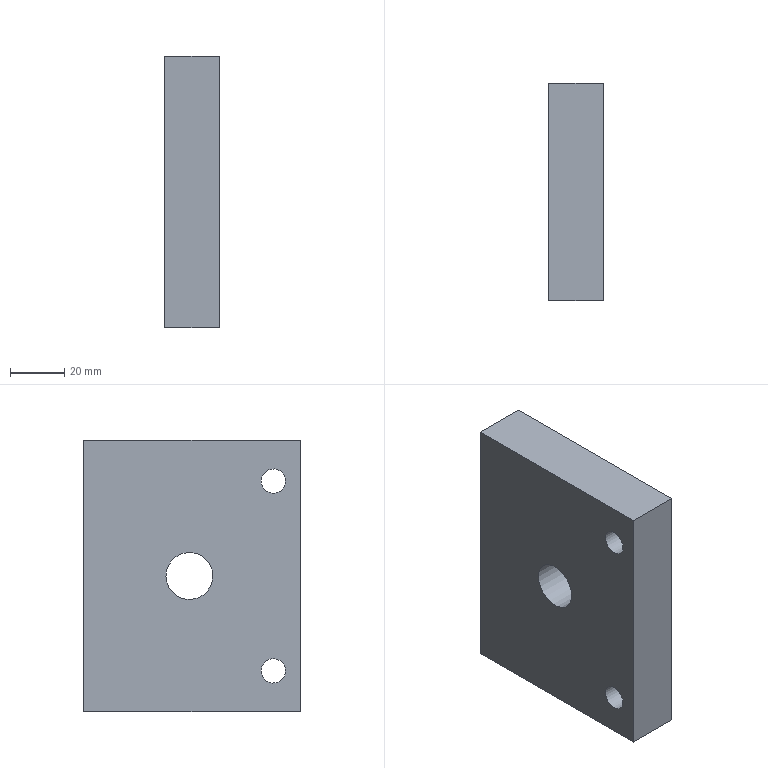Part | STEP file | SN10_001_004_PLACA | 1 solid | 9 faces | box 20 x 80 x 100 mm | volume 152757 mm3 | plane 6 | cylinder 3 | commonest cylinder face diameters 9 x2 17.294 x1
STEP:
#1=CARTESIAN_POINT('',(0.,0.,0.));
#2=DIRECTION('',(0.,0.,1.));
#3=DIRECTION('',(1.,0.,0.));
#4=AXIS2_PLACEMENT_3D('',#1,#2,#3);
#5=CARTESIAN_POINT('',(320.,193.949,32.843));
#6=VERTEX_POINT('',#5);
#7=CARTESIAN_POINT('',(320.,190.,35.));
#8=DIRECTION('',(-1.,0.,0.));
#9=DIRECTION('',(0.,1.,0.));
#10=AXIS2_PLACEMENT_3D('',#7,#8,#9);
#11=CIRCLE('',#10,4.5);
#12=CARTESIAN_POINT('',(319.9,190.,35.));
#13=DIRECTION('',(-1.,0.,0.));
#14=DIRECTION('',(0.,0.8776,-0.4794));
#15=AXIS2_PLACEMENT_3D('',#12,#13,#14);
#16=CYLINDRICAL_SURFACE('',#15,4.5);
#17=CARTESIAN_POINT('',(-0.5,-0.1));
#18=DIRECTION('',(1.,0.));
#19=VECTOR('',#18,1.);
#20=LINE('',#17,#19);
#21=(GEOMETRIC_REPRESENTATION_CONTEXT(2)PARAMETRIC_REPRESENTATION_CONTEXT()REPRESENTATION_CONTEXT('',''));
#22=DEFINITIONAL_REPRESENTATION('',(#20),#21);
#23=PCURVE('',#16,#22);
#24=CARTESIAN_POINT('',(320.,180.,0.));
#25=DIRECTION('',(1.,0.,0.));
#26=DIRECTION('',(0.,0.,-1.));
#27=AXIS2_PLACEMENT_3D('',#24,#25,#26);
#28=PLANE('',#27);
#29=CARTESIAN_POINT('',(-35.,14.5));
#30=CARTESIAN_POINT('',(-27.206,14.5));
#31=CARTESIAN_POINT('',(-31.103,7.75));
#32=CARTESIAN_POINT('',(-35.,1.));
#33=CARTESIAN_POINT('',(-38.897,7.75));
#34=CARTESIAN_POINT('',(-42.794,14.5));
#35=CARTESIAN_POINT('',(-35.,14.5));
#36=(BOUNDED_CURVE()B_SPLINE_CURVE(2,(#29,#30,#31,#32,#33,#34,#35),.UNSPECIFIED.,.T.,.F.)B_SPLINE_CURVE_WITH_KNOTS((1,2,2,2,2,1),(-2.094,0.,2.094,4.189,6.283,8.378),.UNSPECIFIED.)CURVE()GEOMETRIC_REPRESENTATION_ITEM()RATIONAL_B_SPLINE_CURVE((1.,0.5,1.,0.5,1.,0.5,1.))REPRESENTATION_ITEM(''));
#37=(GEOMETRIC_REPRESENTATION_CONTEXT(2)PARAMETRIC_REPRESENTATION_CONTEXT()REPRESENTATION_CONTEXT('',''));
#38=DEFINITIONAL_REPRESENTATION('',(#36),#37);
#39=PCURVE('',#28,#38);
#40=SURFACE_CURVE('',#11,(#23,#39),.PCURVE_S1.);
#41=EDGE_CURVE('',#6,#6,#40,.T.);
#42=ORIENTED_EDGE('',*,*,#41,.T.);
#43=CARTESIAN_POINT('',(300.,193.949,32.843));
#44=VERTEX_POINT('',#43);
#45=CARTESIAN_POINT('',(320.,193.949,32.843));
#46=CARTESIAN_POINT('',(300.,193.949,32.843));
#47=B_SPLINE_CURVE_WITH_KNOTS('',1,(#45,#46),.UNSPECIFIED.,.F.,.F.,(2,2),(-0.1,19.9),.PIECEWISE_BEZIER_KNOTS.);
#48=CARTESIAN_POINT('',(6.283,0.));
#49=DIRECTION('',(0.,1.));
#50=VECTOR('',#49,1.);
#51=LINE('',#48,#50);
#52=(GEOMETRIC_REPRESENTATION_CONTEXT(2)PARAMETRIC_REPRESENTATION_CONTEXT()REPRESENTATION_CONTEXT('',''));
#53=DEFINITIONAL_REPRESENTATION('',(#51),#52);
#54=PCURVE('',#16,#53);
#55=CARTESIAN_POINT('',(0.,0.));
#56=DIRECTION('',(0.,1.));
#57=VECTOR('',#56,1.);
#58=LINE('',#55,#57);
#59=(GEOMETRIC_REPRESENTATION_CONTEXT(2)PARAMETRIC_REPRESENTATION_CONTEXT()REPRESENTATION_CONTEXT('',''));
#60=DEFINITIONAL_REPRESENTATION('',(#58),#59);
#61=PCURVE('',#16,#60);
#62=SEAM_CURVE('',#47,(#54,#61),.PCURVE_S1.);
#63=EDGE_CURVE('',#6,#44,#62,.T.);
#64=ORIENTED_EDGE('',*,*,#63,.T.);
#65=CARTESIAN_POINT('',(300.,190.,35.));
#66=DIRECTION('',(-1.,0.,0.));
#67=DIRECTION('',(0.,1.,0.));
#68=AXIS2_PLACEMENT_3D('',#65,#66,#67);
#69=CIRCLE('',#68,4.5);
#70=CARTESIAN_POINT('',(-0.5,19.9));
#71=DIRECTION('',(1.,0.));
#72=VECTOR('',#71,1.);
#73=LINE('',#70,#72);
#74=(GEOMETRIC_REPRESENTATION_CONTEXT(2)PARAMETRIC_REPRESENTATION_CONTEXT()REPRESENTATION_CONTEXT('',''));
#75=DEFINITIONAL_REPRESENTATION('',(#73),#74);
#76=PCURVE('',#16,#75);
#77=CARTESIAN_POINT('',(300.,260.,0.));
#78=DIRECTION('',(-1.,0.,0.));
#79=DIRECTION('',(0.,0.,1.));
#80=AXIS2_PLACEMENT_3D('',#77,#78,#79);
#81=PLANE('',#80);
#82=CARTESIAN_POINT('',(35.,-70.));
#83=DIRECTION('',(0.,1.));
#84=AXIS2_PLACEMENT_2D('',#82,#83);
#85=CIRCLE('',#84,4.5);
#86=(GEOMETRIC_REPRESENTATION_CONTEXT(2)PARAMETRIC_REPRESENTATION_CONTEXT()REPRESENTATION_CONTEXT('',''));
#87=DEFINITIONAL_REPRESENTATION('',(#85),#86);
#88=PCURVE('',#81,#87);
#89=SURFACE_CURVE('',#69,(#76,#88),.PCURVE_S1.);
#90=EDGE_CURVE('',#44,#44,#89,.T.);
#91=ORIENTED_EDGE('',*,*,#90,.F.);
#92=ORIENTED_EDGE('',*,*,#63,.F.);
#93=EDGE_LOOP('',(#42,#64,#91,#92));
#94=FACE_BOUND('',#93,.F.);
#95=ADVANCED_FACE('',(#94),#16,.F.);
#96=CARTESIAN_POINT('',(320.,260.,-50.));
#97=VERTEX_POINT('',#96);
#98=CARTESIAN_POINT('',(300.,260.,-50.));
#99=VERTEX_POINT('',#98);
#100=CARTESIAN_POINT('',(320.,260.,-50.));
#101=DIRECTION('',(-1.,0.,0.));
#102=VECTOR('',#101,1.);
#103=LINE('',#100,#102);
#104=CARTESIAN_POINT('',(0.,0.,-50.));
#105=DIRECTION('',(0.,0.,1.));
#106=DIRECTION('',(1.,0.,0.));
#107=AXIS2_PLACEMENT_3D('',#104,#105,#106);
#108=PLANE('',#107);
#109=CARTESIAN_POINT('',(320.,260.));
#110=DIRECTION('',(-1.,0.));
#111=VECTOR('',#110,1.);
#112=LINE('',#109,#111);
#113=(GEOMETRIC_REPRESENTATION_CONTEXT(2)PARAMETRIC_REPRESENTATION_CONTEXT()REPRESENTATION_CONTEXT('',''));
#114=DEFINITIONAL_REPRESENTATION('',(#112),#113);
#115=PCURVE('',#108,#114);
#116=CARTESIAN_POINT('',(320.,260.,0.));
#117=DIRECTION('',(0.,1.,0.));
#118=DIRECTION('',(0.,0.,1.));
#119=AXIS2_PLACEMENT_3D('',#116,#117,#118);
#120=PLANE('',#119);
#121=CARTESIAN_POINT('',(-50.,0.));
#122=DIRECTION('',(0.,-1.));
#123=VECTOR('',#122,1.);
#124=LINE('',#121,#123);
#125=(GEOMETRIC_REPRESENTATION_CONTEXT(2)PARAMETRIC_REPRESENTATION_CONTEXT()REPRESENTATION_CONTEXT('',''));
#126=DEFINITIONAL_REPRESENTATION('',(#124),#125);
#127=PCURVE('',#120,#126);
#128=SURFACE_CURVE('',#103,(#115,#127),.PCURVE_S1.);
#129=EDGE_CURVE('',#97,#99,#128,.T.);
#130=ORIENTED_EDGE('',*,*,#129,.F.);
#131=CARTESIAN_POINT('',(320.,180.,-50.));
#132=VERTEX_POINT('',#131);
#133=CARTESIAN_POINT('',(320.,180.,-50.));
#134=DIRECTION('',(0.,1.,0.));
#135=VECTOR('',#134,1.);
#136=LINE('',#133,#135);
#137=CARTESIAN_POINT('',(320.,180.));
#138=DIRECTION('',(0.,1.));
#139=VECTOR('',#138,1.);
#140=LINE('',#137,#139);
#141=(GEOMETRIC_REPRESENTATION_CONTEXT(2)PARAMETRIC_REPRESENTATION_CONTEXT()REPRESENTATION_CONTEXT('',''));
#142=DEFINITIONAL_REPRESENTATION('',(#140),#141);
#143=PCURVE('',#108,#142);
#144=CARTESIAN_POINT('',(50.,0.));
#145=DIRECTION('',(0.,1.));
#146=VECTOR('',#145,1.);
#147=LINE('',#144,#146);
#148=(GEOMETRIC_REPRESENTATION_CONTEXT(2)PARAMETRIC_REPRESENTATION_CONTEXT()REPRESENTATION_CONTEXT('',''));
#149=DEFINITIONAL_REPRESENTATION('',(#147),#148);
#150=PCURVE('',#28,#149);
#151=SURFACE_CURVE('',#136,(#143,#150),.PCURVE_S1.);
#152=EDGE_CURVE('',#132,#97,#151,.T.);
#153=ORIENTED_EDGE('',*,*,#152,.F.);
#154=CARTESIAN_POINT('',(300.,180.,-50.));
#155=VERTEX_POINT('',#154);
#156=CARTESIAN_POINT('',(300.,180.,-50.));
#157=DIRECTION('',(1.,0.,0.));
#158=VECTOR('',#157,1.);
#159=LINE('',#156,#158);
#160=CARTESIAN_POINT('',(300.,180.));
#161=DIRECTION('',(1.,0.));
#162=VECTOR('',#161,1.);
#163=LINE('',#160,#162);
#164=(GEOMETRIC_REPRESENTATION_CONTEXT(2)PARAMETRIC_REPRESENTATION_CONTEXT()REPRESENTATION_CONTEXT('',''));
#165=DEFINITIONAL_REPRESENTATION('',(#163),#164);
#166=PCURVE('',#108,#165);
#167=CARTESIAN_POINT('',(300.,180.,0.));
#168=DIRECTION('',(0.,-1.,0.));
#169=DIRECTION('',(0.,0.,-1.));
#170=AXIS2_PLACEMENT_3D('',#167,#168,#169);
#171=PLANE('',#170);
#172=CARTESIAN_POINT('',(50.,0.));
#173=DIRECTION('',(0.,1.));
#174=VECTOR('',#173,1.);
#175=LINE('',#172,#174);
#176=(GEOMETRIC_REPRESENTATION_CONTEXT(2)PARAMETRIC_REPRESENTATION_CONTEXT()REPRESENTATION_CONTEXT('',''));
#177=DEFINITIONAL_REPRESENTATION('',(#175),#176);
#178=PCURVE('',#171,#177);
#179=SURFACE_CURVE('',#159,(#166,#178),.PCURVE_S1.);
#180=EDGE_CURVE('',#155,#132,#179,.T.);
#181=ORIENTED_EDGE('',*,*,#180,.F.);
#182=CARTESIAN_POINT('',(300.,260.,-50.));
#183=DIRECTION('',(0.,-1.,0.));
#184=VECTOR('',#183,1.);
#185=LINE('',#182,#184);
#186=CARTESIAN_POINT('',(300.,260.));
#187=DIRECTION('',(0.,-1.));
#188=VECTOR('',#187,1.);
#189=LINE('',#186,#188);
#190=(GEOMETRIC_REPRESENTATION_CONTEXT(2)PARAMETRIC_REPRESENTATION_CONTEXT()REPRESENTATION_CONTEXT('',''));
#191=DEFINITIONAL_REPRESENTATION('',(#189),#190);
#192=PCURVE('',#108,#191);
#193=CARTESIAN_POINT('',(-50.,0.));
#194=DIRECTION('',(0.,-1.));
#195=VECTOR('',#194,1.);
#196=LINE('',#193,#195);
#197=(GEOMETRIC_REPRESENTATION_CONTEXT(2)PARAMETRIC_REPRESENTATION_CONTEXT()REPRESENTATION_CONTEXT('',''));
#198=DEFINITIONAL_REPRESENTATION('',(#196),#197);
#199=PCURVE('',#81,#198);
#200=SURFACE_CURVE('',#185,(#192,#199),.PCURVE_S1.);
#201=EDGE_CURVE('',#99,#155,#200,.T.);
#202=ORIENTED_EDGE('',*,*,#201,.F.);
#203=EDGE_LOOP('',(#130,#153,#181,#202));
#204=FACE_BOUND('',#203,.T.);
#205=ADVANCED_FACE('',(#204),#108,.F.);
#206=CARTESIAN_POINT('',(320.,260.,50.));
#207=VERTEX_POINT('',#206);
#208=CARTESIAN_POINT('',(320.,260.,-50.));
#209=DIRECTION('',(0.,0.,1.));
#210=VECTOR('',#209,1.);
#211=LINE('',#208,#210);
#212=CARTESIAN_POINT('',(-50.,0.));
#213=DIRECTION('',(1.,0.));
#214=VECTOR('',#213,1.);
#215=LINE('',#212,#214);
#216=(GEOMETRIC_REPRESENTATION_CONTEXT(2)PARAMETRIC_REPRESENTATION_CONTEXT()REPRESENTATION_CONTEXT('',''));
#217=DEFINITIONAL_REPRESENTATION('',(#215),#216);
#218=PCURVE('',#120,#217);
#219=CARTESIAN_POINT('',(50.,80.));
#220=DIRECTION('',(-1.,0.));
#221=VECTOR('',#220,1.);
#222=LINE('',#219,#221);
#223=(GEOMETRIC_REPRESENTATION_CONTEXT(2)PARAMETRIC_REPRESENTATION_CONTEXT()REPRESENTATION_CONTEXT('',''));
#224=DEFINITIONAL_REPRESENTATION('',(#222),#223);
#225=PCURVE('',#28,#224);
#226=SURFACE_CURVE('',#211,(#218,#225),.PCURVE_S1.);
#227=EDGE_CURVE('',#97,#207,#226,.T.);
#228=ORIENTED_EDGE('',*,*,#227,.F.);
#229=ORIENTED_EDGE('',*,*,#129,.T.);
#230=CARTESIAN_POINT('',(300.,260.,50.));
#231=VERTEX_POINT('',#230);
#232=CARTESIAN_POINT('',(300.,260.,-50.));
#233=DIRECTION('',(0.,0.,1.));
#234=VECTOR('',#233,1.);
#235=LINE('',#232,#234);
#236=CARTESIAN_POINT('',(-50.,-20.));
#237=DIRECTION('',(1.,0.));
#238=VECTOR('',#237,1.);
#239=LINE('',#236,#238);
#240=(GEOMETRIC_REPRESENTATION_CONTEXT(2)PARAMETRIC_REPRESENTATION_CONTEXT()REPRESENTATION_CONTEXT('',''));
#241=DEFINITIONAL_REPRESENTATION('',(#239),#240);
#242=PCURVE('',#120,#241);
#243=CARTESIAN_POINT('',(-50.,0.));
#244=DIRECTION('',(1.,0.));
#245=VECTOR('',#244,1.);
#246=LINE('',#243,#245);
#247=(GEOMETRIC_REPRESENTATION_CONTEXT(2)PARAMETRIC_REPRESENTATION_CONTEXT()REPRESENTATION_CONTEXT('',''));
#248=DEFINITIONAL_REPRESENTATION('',(#246),#247);
#249=PCURVE('',#81,#248);
#250=SURFACE_CURVE('',#235,(#242,#249),.PCURVE_S1.);
#251=EDGE_CURVE('',#99,#231,#250,.T.);
#252=ORIENTED_EDGE('',*,*,#251,.T.);
#253=CARTESIAN_POINT('',(320.,260.,50.));
#254=DIRECTION('',(-1.,0.,0.));
#255=VECTOR('',#254,1.);
#256=LINE('',#253,#255);
#257=CARTESIAN_POINT('',(50.,0.));
#258=DIRECTION('',(0.,-1.));
#259=VECTOR('',#258,1.);
#260=LINE('',#257,#259);
#261=(GEOMETRIC_REPRESENTATION_CONTEXT(2)PARAMETRIC_REPRESENTATION_CONTEXT()REPRESENTATION_CONTEXT('',''));
#262=DEFINITIONAL_REPRESENTATION('',(#260),#261);
#263=PCURVE('',#120,#262);
#264=CARTESIAN_POINT('',(0.,0.,50.));
#265=DIRECTION('',(0.,0.,1.));
#266=DIRECTION('',(1.,0.,0.));
#267=AXIS2_PLACEMENT_3D('',#264,#265,#266);
#268=PLANE('',#267);
#269=CARTESIAN_POINT('',(320.,260.));
#270=DIRECTION('',(-1.,0.));
#271=VECTOR('',#270,1.);
#272=LINE('',#269,#271);
#273=(GEOMETRIC_REPRESENTATION_CONTEXT(2)PARAMETRIC_REPRESENTATION_CONTEXT()REPRESENTATION_CONTEXT('',''));
#274=DEFINITIONAL_REPRESENTATION('',(#272),#273);
#275=PCURVE('',#268,#274);
#276=SURFACE_CURVE('',#256,(#263,#275),.PCURVE_S1.);
#277=EDGE_CURVE('',#207,#231,#276,.T.);
#278=ORIENTED_EDGE('',*,*,#277,.F.);
#279=EDGE_LOOP('',(#228,#229,#252,#278));
#280=FACE_BOUND('',#279,.T.);
#281=ADVANCED_FACE('',(#280),#120,.T.);
#282=CARTESIAN_POINT('',(320.,228.538,-4.146));
#283=VERTEX_POINT('',#282);
#284=CARTESIAN_POINT('',(320.,220.95,0.));
#285=DIRECTION('',(-1.,0.,0.));
#286=DIRECTION('',(0.,1.,0.));
#287=AXIS2_PLACEMENT_3D('',#284,#285,#286);
#288=CIRCLE('',#287,8.647);
#289=CARTESIAN_POINT('',(319.9,220.95,0.));
#290=DIRECTION('',(-1.,0.,0.));
#291=DIRECTION('',(0.,0.8776,-0.4794));
#292=AXIS2_PLACEMENT_3D('',#289,#290,#291);
#293=CYLINDRICAL_SURFACE('',#292,8.647);
#294=CARTESIAN_POINT('',(-0.5,-0.1));
#295=DIRECTION('',(1.,0.));
#296=VECTOR('',#295,1.);
#297=LINE('',#294,#296);
#298=(GEOMETRIC_REPRESENTATION_CONTEXT(2)PARAMETRIC_REPRESENTATION_CONTEXT()REPRESENTATION_CONTEXT('',''));
#299=DEFINITIONAL_REPRESENTATION('',(#297),#298);
#300=PCURVE('',#293,#299);
#301=CARTESIAN_POINT('',(0.,49.597));
#302=CARTESIAN_POINT('',(14.977,49.597));
#303=CARTESIAN_POINT('',(7.489,36.627));
#304=CARTESIAN_POINT('',(0.,23.656));
#305=CARTESIAN_POINT('',(-7.489,36.627));
#306=CARTESIAN_POINT('',(-14.977,49.597));
#307=CARTESIAN_POINT('',(0.,49.597));
#308=(BOUNDED_CURVE()B_SPLINE_CURVE(2,(#301,#302,#303,#304,#305,#306,#307),.UNSPECIFIED.,.T.,.F.)B_SPLINE_CURVE_WITH_KNOTS((1,2,2,2,2,1),(-2.094,0.,2.094,4.189,6.283,8.378),.UNSPECIFIED.)CURVE()GEOMETRIC_REPRESENTATION_ITEM()RATIONAL_B_SPLINE_CURVE((1.,0.5,1.,0.5,1.,0.5,1.))REPRESENTATION_ITEM(''));
#309=(GEOMETRIC_REPRESENTATION_CONTEXT(2)PARAMETRIC_REPRESENTATION_CONTEXT()REPRESENTATION_CONTEXT('',''));
#310=DEFINITIONAL_REPRESENTATION('',(#308),#309);
#311=PCURVE('',#28,#310);
#312=SURFACE_CURVE('',#288,(#300,#311),.PCURVE_S1.);
#313=EDGE_CURVE('',#283,#283,#312,.T.);
#314=ORIENTED_EDGE('',*,*,#313,.T.);
#315=CARTESIAN_POINT('',(300.,228.538,-4.146));
#316=VERTEX_POINT('',#315);
#317=CARTESIAN_POINT('',(320.,228.538,-4.146));
#318=CARTESIAN_POINT('',(300.,228.538,-4.146));
#319=B_SPLINE_CURVE_WITH_KNOTS('',1,(#317,#318),.UNSPECIFIED.,.F.,.F.,(2,2),(-0.1,19.9),.PIECEWISE_BEZIER_KNOTS.);
#320=CARTESIAN_POINT('',(6.283,0.));
#321=DIRECTION('',(0.,1.));
#322=VECTOR('',#321,1.);
#323=LINE('',#320,#322);
#324=(GEOMETRIC_REPRESENTATION_CONTEXT(2)PARAMETRIC_REPRESENTATION_CONTEXT()REPRESENTATION_CONTEXT('',''));
#325=DEFINITIONAL_REPRESENTATION('',(#323),#324);
#326=PCURVE('',#293,#325);
#327=CARTESIAN_POINT('',(0.,0.));
#328=DIRECTION('',(0.,1.));
#329=VECTOR('',#328,1.);
#330=LINE('',#327,#329);
#331=(GEOMETRIC_REPRESENTATION_CONTEXT(2)PARAMETRIC_REPRESENTATION_CONTEXT()REPRESENTATION_CONTEXT('',''));
#332=DEFINITIONAL_REPRESENTATION('',(#330),#331);
#333=PCURVE('',#293,#332);
#334=SEAM_CURVE('',#319,(#326,#333),.PCURVE_S1.);
#335=EDGE_CURVE('',#283,#316,#334,.T.);
#336=ORIENTED_EDGE('',*,*,#335,.T.);
#337=CARTESIAN_POINT('',(300.,220.95,0.));
#338=DIRECTION('',(-1.,0.,0.));
#339=DIRECTION('',(0.,1.,0.));
#340=AXIS2_PLACEMENT_3D('',#337,#338,#339);
#341=CIRCLE('',#340,8.647);
#342=CARTESIAN_POINT('',(-0.5,19.9));
#343=DIRECTION('',(1.,0.));
#344=VECTOR('',#343,1.);
#345=LINE('',#342,#344);
#346=(GEOMETRIC_REPRESENTATION_CONTEXT(2)PARAMETRIC_REPRESENTATION_CONTEXT()REPRESENTATION_CONTEXT('',''));
#347=DEFINITIONAL_REPRESENTATION('',(#345),#346);
#348=PCURVE('',#293,#347);
#349=CARTESIAN_POINT('',(0.,-39.05));
#350=DIRECTION('',(0.,1.));
#351=AXIS2_PLACEMENT_2D('',#349,#350);
#352=CIRCLE('',#351,8.647);
#353=(GEOMETRIC_REPRESENTATION_CONTEXT(2)PARAMETRIC_REPRESENTATION_CONTEXT()REPRESENTATION_CONTEXT('',''));
#354=DEFINITIONAL_REPRESENTATION('',(#352),#353);
#355=PCURVE('',#81,#354);
#356=SURFACE_CURVE('',#341,(#348,#355),.PCURVE_S1.);
#357=EDGE_CURVE('',#316,#316,#356,.T.);
#358=ORIENTED_EDGE('',*,*,#357,.F.);
#359=ORIENTED_EDGE('',*,*,#335,.F.);
#360=EDGE_LOOP('',(#314,#336,#358,#359));
#361=FACE_BOUND('',#360,.F.);
#362=ADVANCED_FACE('',(#361),#293,.F.);
#363=CARTESIAN_POINT('',(300.,180.,50.));
#364=VERTEX_POINT('',#363);
#365=CARTESIAN_POINT('',(300.,260.,50.));
#366=DIRECTION('',(0.,-1.,0.));
#367=VECTOR('',#366,1.);
#368=LINE('',#365,#367);
#369=CARTESIAN_POINT('',(300.,260.));
#370=DIRECTION('',(0.,-1.));
#371=VECTOR('',#370,1.);
#372=LINE('',#369,#371);
#373=(GEOMETRIC_REPRESENTATION_CONTEXT(2)PARAMETRIC_REPRESENTATION_CONTEXT()REPRESENTATION_CONTEXT('',''));
#374=DEFINITIONAL_REPRESENTATION('',(#372),#373);
#375=PCURVE('',#268,#374);
#376=CARTESIAN_POINT('',(50.,0.));
#377=DIRECTION('',(0.,-1.));
#378=VECTOR('',#377,1.);
#379=LINE('',#376,#378);
#380=(GEOMETRIC_REPRESENTATION_CONTEXT(2)PARAMETRIC_REPRESENTATION_CONTEXT()REPRESENTATION_CONTEXT('',''));
#381=DEFINITIONAL_REPRESENTATION('',(#379),#380);
#382=PCURVE('',#81,#381);
#383=SURFACE_CURVE('',#368,(#375,#382),.PCURVE_S1.);
#384=EDGE_CURVE('',#231,#364,#383,.T.);
#385=ORIENTED_EDGE('',*,*,#384,.T.);
#386=CARTESIAN_POINT('',(320.,180.,50.));
#387=VERTEX_POINT('',#386);
#388=CARTESIAN_POINT('',(300.,180.,50.));
#389=DIRECTION('',(1.,0.,0.));
#390=VECTOR('',#389,1.);
#391=LINE('',#388,#390);
#392=CARTESIAN_POINT('',(300.,180.));
#393=DIRECTION('',(1.,0.));
#394=VECTOR('',#393,1.);
#395=LINE('',#392,#394);
#396=(GEOMETRIC_REPRESENTATION_CONTEXT(2)PARAMETRIC_REPRESENTATION_CONTEXT()REPRESENTATION_CONTEXT('',''));
#397=DEFINITIONAL_REPRESENTATION('',(#395),#396);
#398=PCURVE('',#268,#397);
#399=CARTESIAN_POINT('',(-50.,0.));
#400=DIRECTION('',(0.,1.));
#401=VECTOR('',#400,1.);
#402=LINE('',#399,#401);
#403=(GEOMETRIC_REPRESENTATION_CONTEXT(2)PARAMETRIC_REPRESENTATION_CONTEXT()REPRESENTATION_CONTEXT('',''));
#404=DEFINITIONAL_REPRESENTATION('',(#402),#403);
#405=PCURVE('',#171,#404);
#406=SURFACE_CURVE('',#391,(#398,#405),.PCURVE_S1.);
#407=EDGE_CURVE('',#364,#387,#406,.T.);
#408=ORIENTED_EDGE('',*,*,#407,.T.);
#409=CARTESIAN_POINT('',(320.,180.,50.));
#410=DIRECTION('',(0.,1.,0.));
#411=VECTOR('',#410,1.);
#412=LINE('',#409,#411);
#413=CARTESIAN_POINT('',(320.,180.));
#414=DIRECTION('',(0.,1.));
#415=VECTOR('',#414,1.);
#416=LINE('',#413,#415);
#417=(GEOMETRIC_REPRESENTATION_CONTEXT(2)PARAMETRIC_REPRESENTATION_CONTEXT()REPRESENTATION_CONTEXT('',''));
#418=DEFINITIONAL_REPRESENTATION('',(#416),#417);
#419=PCURVE('',#268,#418);
#420=CARTESIAN_POINT('',(-50.,0.));
#421=DIRECTION('',(0.,1.));
#422=VECTOR('',#421,1.);
#423=LINE('',#420,#422);
#424=(GEOMETRIC_REPRESENTATION_CONTEXT(2)PARAMETRIC_REPRESENTATION_CONTEXT()REPRESENTATION_CONTEXT('',''));
#425=DEFINITIONAL_REPRESENTATION('',(#423),#424);
#426=PCURVE('',#28,#425);
#427=SURFACE_CURVE('',#412,(#419,#426),.PCURVE_S1.);
#428=EDGE_CURVE('',#387,#207,#427,.T.);
#429=ORIENTED_EDGE('',*,*,#428,.T.);
#430=ORIENTED_EDGE('',*,*,#277,.T.);
#431=EDGE_LOOP('',(#385,#408,#429,#430));
#432=FACE_BOUND('',#431,.T.);
#433=ADVANCED_FACE('',(#432),#268,.T.);
#434=CARTESIAN_POINT('',(300.,180.,-50.));
#435=DIRECTION('',(0.,0.,1.));
#436=VECTOR('',#435,1.);
#437=LINE('',#434,#436);
#438=CARTESIAN_POINT('',(50.,0.));
#439=DIRECTION('',(-1.,0.));
#440=VECTOR('',#439,1.);
#441=LINE('',#438,#440);
#442=(GEOMETRIC_REPRESENTATION_CONTEXT(2)PARAMETRIC_REPRESENTATION_CONTEXT()REPRESENTATION_CONTEXT('',''));
#443=DEFINITIONAL_REPRESENTATION('',(#441),#442);
#444=PCURVE('',#171,#443);
#445=CARTESIAN_POINT('',(-50.,-80.));
#446=DIRECTION('',(1.,0.));
#447=VECTOR('',#446,1.);
#448=LINE('',#445,#447);
#449=(GEOMETRIC_REPRESENTATION_CONTEXT(2)PARAMETRIC_REPRESENTATION_CONTEXT()REPRESENTATION_CONTEXT('',''));
#450=DEFINITIONAL_REPRESENTATION('',(#448),#449);
#451=PCURVE('',#81,#450);
#452=SURFACE_CURVE('',#437,(#444,#451),.PCURVE_S1.);
#453=EDGE_CURVE('',#155,#364,#452,.T.);
#454=ORIENTED_EDGE('',*,*,#453,.F.);
#455=ORIENTED_EDGE('',*,*,#180,.T.);
#456=CARTESIAN_POINT('',(320.,180.,-50.));
#457=DIRECTION('',(0.,0.,1.));
#458=VECTOR('',#457,1.);
#459=LINE('',#456,#458);
#460=CARTESIAN_POINT('',(50.,20.));
#461=DIRECTION('',(-1.,0.));
#462=VECTOR('',#461,1.);
#463=LINE('',#460,#462);
#464=(GEOMETRIC_REPRESENTATION_CONTEXT(2)PARAMETRIC_REPRESENTATION_CONTEXT()REPRESENTATION_CONTEXT('',''));
#465=DEFINITIONAL_REPRESENTATION('',(#463),#464);
#466=PCURVE('',#171,#465);
#467=CARTESIAN_POINT('',(50.,0.));
#468=DIRECTION('',(-1.,0.));
#469=VECTOR('',#468,1.);
#470=LINE('',#467,#469);
#471=(GEOMETRIC_REPRESENTATION_CONTEXT(2)PARAMETRIC_REPRESENTATION_CONTEXT()REPRESENTATION_CONTEXT('',''));
#472=DEFINITIONAL_REPRESENTATION('',(#470),#471);
#473=PCURVE('',#28,#472);
#474=SURFACE_CURVE('',#459,(#466,#473),.PCURVE_S1.);
#475=EDGE_CURVE('',#132,#387,#474,.T.);
#476=ORIENTED_EDGE('',*,*,#475,.T.);
#477=ORIENTED_EDGE('',*,*,#407,.F.);
#478=EDGE_LOOP('',(#454,#455,#476,#477));
#479=FACE_BOUND('',#478,.T.);
#480=ADVANCED_FACE('',(#479),#171,.T.);
#481=ORIENTED_EDGE('',*,*,#251,.F.);
#482=ORIENTED_EDGE('',*,*,#201,.T.);
#483=ORIENTED_EDGE('',*,*,#453,.T.);
#484=ORIENTED_EDGE('',*,*,#384,.F.);
#485=EDGE_LOOP('',(#481,#482,#483,#484));
#486=FACE_BOUND('',#485,.T.);
#487=CARTESIAN_POINT('',(300.,193.949,-37.157));
#488=VERTEX_POINT('',#487);
#489=CARTESIAN_POINT('',(300.,190.,-35.));
#490=DIRECTION('',(-1.,0.,0.));
#491=DIRECTION('',(0.,1.,0.));
#492=AXIS2_PLACEMENT_3D('',#489,#490,#491);
#493=CIRCLE('',#492,4.5);
#494=CARTESIAN_POINT('',(-35.,-70.));
#495=DIRECTION('',(0.,1.));
#496=AXIS2_PLACEMENT_2D('',#494,#495);
#497=CIRCLE('',#496,4.5);
#498=(GEOMETRIC_REPRESENTATION_CONTEXT(2)PARAMETRIC_REPRESENTATION_CONTEXT()REPRESENTATION_CONTEXT('',''));
#499=DEFINITIONAL_REPRESENTATION('',(#497),#498);
#500=PCURVE('',#81,#499);
#501=CARTESIAN_POINT('',(319.9,190.,-35.));
#502=DIRECTION('',(-1.,0.,0.));
#503=DIRECTION('',(0.,0.8776,-0.4794));
#504=AXIS2_PLACEMENT_3D('',#501,#502,#503);
#505=CYLINDRICAL_SURFACE('',#504,4.5);
#506=CARTESIAN_POINT('',(-0.5,19.9));
#507=DIRECTION('',(1.,0.));
#508=VECTOR('',#507,1.);
#509=LINE('',#506,#508);
#510=(GEOMETRIC_REPRESENTATION_CONTEXT(2)PARAMETRIC_REPRESENTATION_CONTEXT()REPRESENTATION_CONTEXT('',''));
#511=DEFINITIONAL_REPRESENTATION('',(#509),#510);
#512=PCURVE('',#505,#511);
#513=SURFACE_CURVE('',#493,(#500,#512),.PCURVE_S1.);
#514=EDGE_CURVE('',#488,#488,#513,.T.);
#515=ORIENTED_EDGE('',*,*,#514,.F.);
#516=EDGE_LOOP('',(#515));
#517=FACE_BOUND('',#516,.T.);
#518=ORIENTED_EDGE('',*,*,#90,.F.);
#519=EDGE_LOOP('',(#518));
#520=FACE_BOUND('',#519,.T.);
#521=ORIENTED_EDGE('',*,*,#357,.F.);
#522=EDGE_LOOP('',(#521));
#523=FACE_BOUND('',#522,.T.);
#524=ADVANCED_FACE('',(#486,#517,#520,#523),#81,.T.);
#525=ORIENTED_EDGE('',*,*,#475,.F.);
#526=ORIENTED_EDGE('',*,*,#152,.T.);
#527=ORIENTED_EDGE('',*,*,#227,.T.);
#528=ORIENTED_EDGE('',*,*,#428,.F.);
#529=EDGE_LOOP('',(#525,#526,#527,#528));
#530=FACE_BOUND('',#529,.T.);
#531=CARTESIAN_POINT('',(320.,193.949,-37.157));
#532=VERTEX_POINT('',#531);
#533=CARTESIAN_POINT('',(320.,190.,-35.));
#534=DIRECTION('',(1.,0.,0.));
#535=DIRECTION('',(0.,1.,0.));
#536=AXIS2_PLACEMENT_3D('',#533,#534,#535);
#537=CIRCLE('',#536,4.5);
#538=CARTESIAN_POINT('',(35.,10.));
#539=DIRECTION('',(0.,1.));
#540=AXIS2_PLACEMENT_2D('',#538,#539);
#541=CIRCLE('',#540,4.5);
#542=(GEOMETRIC_REPRESENTATION_CONTEXT(2)PARAMETRIC_REPRESENTATION_CONTEXT()REPRESENTATION_CONTEXT('',''));
#543=DEFINITIONAL_REPRESENTATION('',(#541),#542);
#544=PCURVE('',#28,#543);
#545=CARTESIAN_POINT('',(12.066,-0.1));
#546=DIRECTION('',(-1.,0.));
#547=VECTOR('',#546,1.);
#548=LINE('',#545,#547);
#549=(GEOMETRIC_REPRESENTATION_CONTEXT(2)PARAMETRIC_REPRESENTATION_CONTEXT()REPRESENTATION_CONTEXT('',''));
#550=DEFINITIONAL_REPRESENTATION('',(#548),#549);
#551=PCURVE('',#505,#550);
#552=SURFACE_CURVE('',#537,(#544,#551),.PCURVE_S1.);
#553=EDGE_CURVE('',#532,#532,#552,.T.);
#554=ORIENTED_EDGE('',*,*,#553,.F.);
#555=EDGE_LOOP('',(#554));
#556=FACE_BOUND('',#555,.T.);
#557=ORIENTED_EDGE('',*,*,#41,.T.);
#558=EDGE_LOOP('',(#557));
#559=FACE_BOUND('',#558,.T.);
#560=ORIENTED_EDGE('',*,*,#313,.T.);
#561=EDGE_LOOP('',(#560));
#562=FACE_BOUND('',#561,.T.);
#563=ADVANCED_FACE('',(#530,#556,#559,#562),#28,.T.);
#564=ORIENTED_EDGE('',*,*,#553,.F.);
#565=CARTESIAN_POINT('',(320.,193.949,-37.157));
#566=CARTESIAN_POINT('',(300.,193.949,-37.157));
#567=B_SPLINE_CURVE_WITH_KNOTS('',1,(#565,#566),.UNSPECIFIED.,.F.,.F.,(2,2),(-0.1,19.9),.PIECEWISE_BEZIER_KNOTS.);
#568=CARTESIAN_POINT('',(6.283,0.));
#569=DIRECTION('',(0.,1.));
#570=VECTOR('',#569,1.);
#571=LINE('',#568,#570);
#572=(GEOMETRIC_REPRESENTATION_CONTEXT(2)PARAMETRIC_REPRESENTATION_CONTEXT()REPRESENTATION_CONTEXT('',''));
#573=DEFINITIONAL_REPRESENTATION('',(#571),#572);
#574=PCURVE('',#505,#573);
#575=CARTESIAN_POINT('',(0.,0.));
#576=DIRECTION('',(0.,1.));
#577=VECTOR('',#576,1.);
#578=LINE('',#575,#577);
#579=(GEOMETRIC_REPRESENTATION_CONTEXT(2)PARAMETRIC_REPRESENTATION_CONTEXT()REPRESENTATION_CONTEXT('',''));
#580=DEFINITIONAL_REPRESENTATION('',(#578),#579);
#581=PCURVE('',#505,#580);
#582=SEAM_CURVE('',#567,(#574,#581),.PCURVE_S1.);
#583=EDGE_CURVE('',#532,#488,#582,.T.);
#584=ORIENTED_EDGE('',*,*,#583,.T.);
#585=ORIENTED_EDGE('',*,*,#514,.F.);
#586=ORIENTED_EDGE('',*,*,#583,.F.);
#587=EDGE_LOOP('',(#564,#584,#585,#586));
#588=FACE_BOUND('',#587,.F.);
#589=ADVANCED_FACE('',(#588),#505,.F.);
#590=CLOSED_SHELL('',(#95,#205,#281,#362,#433,#480,#524,#563,#589));
#591=MANIFOLD_SOLID_BREP('',#590);
#592=(LENGTH_UNIT()NAMED_UNIT(*)SI_UNIT(.MILLI.,.METRE.));
#593=UNCERTAINTY_MEASURE_WITH_UNIT(LENGTH_MEASURE(0.000002),#592,'','');
#594=(NAMED_UNIT(*)PLANE_ANGLE_UNIT()SI_UNIT($,.RADIAN.));
#595=(NAMED_UNIT(*)SI_UNIT($,.STERADIAN.)SOLID_ANGLE_UNIT());
#596=(GEOMETRIC_REPRESENTATION_CONTEXT(3)GLOBAL_UNCERTAINTY_ASSIGNED_CONTEXT((#593))GLOBAL_UNIT_ASSIGNED_CONTEXT((#592,#594,#595))REPRESENTATION_CONTEXT('',''));
#597=ADVANCED_BREP_SHAPE_REPRESENTATION('',(#4,#591),#596);